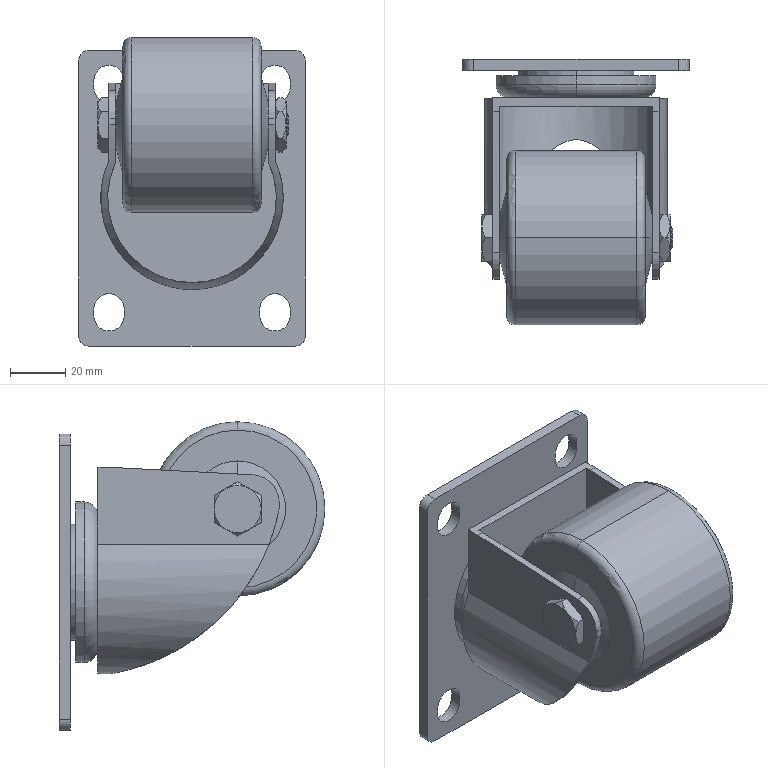Part | STEP file | CGL01-D63 | 3 solids | 117 faces | box 82 x 96 x 111.5 mm | volume 244829 mm3 | plane 49 | cylinder 35 | cone 27 | torus 6 | commonest cylinder face diameters 11 x12 8 x6 20 x2 25 x2 40 x2 42 x2